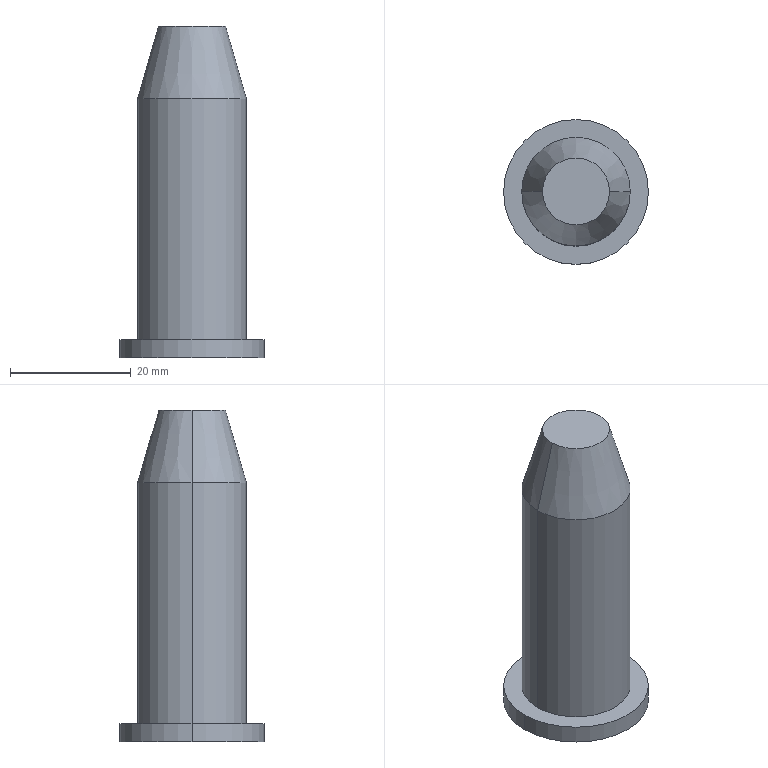Part | STEP file | YCD14007A-08.02.15 Latch Cylinder Joint | 1 solid | 13 faces | box 24 x 24 x 55 mm | volume 9061 mm3 | cylinder 6 | cone 4 | plane 3 | commonest cylinder face diameters 12.5 x2 18 x2 24 x2
STEP:
#1=CARTESIAN_POINT('',(0.,0.,0.));
#2=DIRECTION('',(0.,0.,1.));
#3=DIRECTION('',(1.,0.,0.));
#4=AXIS2_PLACEMENT_3D('',#1,#2,#3);
#5=CARTESIAN_POINT('',(-6.25,0.,35.5));
#6=VERTEX_POINT('',#5);
#7=CARTESIAN_POINT('',(-6.25,0.,0.));
#8=VERTEX_POINT('',#7);
#9=CARTESIAN_POINT('',(-6.25,0.,0.));
#10=DIRECTION('',(0.,0.,-1.));
#11=VECTOR('',#10,1.);
#12=LINE('',#9,#11);
#13=CARTESIAN_POINT('',(0.,0.,0.));
#14=DIRECTION('',(0.,0.,-1.));
#15=DIRECTION('',(-1.,0.,0.));
#16=AXIS2_PLACEMENT_3D('',#13,#14,#15);
#17=CYLINDRICAL_SURFACE('',#16,6.25);
#18=CARTESIAN_POINT('',(6.283,0.));
#19=DIRECTION('',(0.,1.));
#20=VECTOR('',#19,1.);
#21=LINE('',#18,#20);
#22=(GEOMETRIC_REPRESENTATION_CONTEXT(2)PARAMETRIC_REPRESENTATION_CONTEXT()REPRESENTATION_CONTEXT('',''));
#23=DEFINITIONAL_REPRESENTATION('',(#21),#22);
#24=PCURVE('',#17,#23);
#25=CARTESIAN_POINT('',(0.,0.,0.));
#26=DIRECTION('',(0.,0.,-1.));
#27=DIRECTION('',(-1.,0.,0.));
#28=AXIS2_PLACEMENT_3D('',#25,#26,#27);
#29=CYLINDRICAL_SURFACE('',#28,6.25);
#30=CARTESIAN_POINT('',(0.,0.));
#31=DIRECTION('',(0.,1.));
#32=VECTOR('',#31,1.);
#33=LINE('',#30,#32);
#34=(GEOMETRIC_REPRESENTATION_CONTEXT(2)PARAMETRIC_REPRESENTATION_CONTEXT()REPRESENTATION_CONTEXT('',''));
#35=DEFINITIONAL_REPRESENTATION('',(#33),#34);
#36=PCURVE('',#29,#35);
#37=SURFACE_CURVE('',#12,(#24,#36),.PCURVE_S1.);
#38=EDGE_CURVE('',#6,#8,#37,.T.);
#39=ORIENTED_EDGE('',*,*,#38,.T.);
#40=CARTESIAN_POINT('',(6.25,0.,0.));
#41=VERTEX_POINT('',#40);
#42=CARTESIAN_POINT('',(0.,0.,0.));
#43=DIRECTION('',(0.,0.,-1.));
#44=DIRECTION('',(-1.,0.,0.));
#45=AXIS2_PLACEMENT_3D('',#42,#43,#44);
#46=CIRCLE('',#45,6.25);
#47=CARTESIAN_POINT('',(0.,0.));
#48=DIRECTION('',(1.,0.));
#49=VECTOR('',#48,1.);
#50=LINE('',#47,#49);
#51=(GEOMETRIC_REPRESENTATION_CONTEXT(2)PARAMETRIC_REPRESENTATION_CONTEXT()REPRESENTATION_CONTEXT('',''));
#52=DEFINITIONAL_REPRESENTATION('',(#50),#51);
#53=PCURVE('',#17,#52);
#54=CARTESIAN_POINT('',(0.,0.,0.));
#55=DIRECTION('',(0.,0.,1.));
#56=DIRECTION('',(1.,0.,0.));
#57=AXIS2_PLACEMENT_3D('',#54,#55,#56);
#58=PLANE('',#57);
#59=CARTESIAN_POINT('',(-6.25,0.));
#60=CARTESIAN_POINT('',(-6.25,10.825));
#61=CARTESIAN_POINT('',(3.125,5.413));
#62=CARTESIAN_POINT('',(12.5,0.));
#63=CARTESIAN_POINT('',(3.125,-5.413));
#64=CARTESIAN_POINT('',(-6.25,-10.825));
#65=CARTESIAN_POINT('',(-6.25,0.));
#66=(BOUNDED_CURVE()B_SPLINE_CURVE(2,(#59,#60,#61,#62,#63,#64,#65),.UNSPECIFIED.,.T.,.F.)B_SPLINE_CURVE_WITH_KNOTS((1,2,2,2,2,1),(-2.094,0.,2.094,4.189,6.283,8.378),.UNSPECIFIED.)CURVE()GEOMETRIC_REPRESENTATION_ITEM()RATIONAL_B_SPLINE_CURVE((1.,0.5,1.,0.5,1.,0.5,1.))REPRESENTATION_ITEM(''));
#67=(GEOMETRIC_REPRESENTATION_CONTEXT(2)PARAMETRIC_REPRESENTATION_CONTEXT()REPRESENTATION_CONTEXT('',''));
#68=DEFINITIONAL_REPRESENTATION('',(#66),#67);
#69=PCURVE('',#58,#68);
#70=SURFACE_CURVE('',#46,(#53,#69),.PCURVE_S1.);
#71=EDGE_CURVE('',#41,#8,#70,.T.);
#72=ORIENTED_EDGE('',*,*,#71,.F.);
#73=CARTESIAN_POINT('',(6.25,0.,35.5));
#74=VERTEX_POINT('',#73);
#75=CARTESIAN_POINT('',(6.25,0.,0.));
#76=DIRECTION('',(0.,0.,-1.));
#77=VECTOR('',#76,1.);
#78=LINE('',#75,#77);
#79=CARTESIAN_POINT('',(3.142,0.));
#80=DIRECTION('',(0.,1.));
#81=VECTOR('',#80,1.);
#82=LINE('',#79,#81);
#83=(GEOMETRIC_REPRESENTATION_CONTEXT(2)PARAMETRIC_REPRESENTATION_CONTEXT()REPRESENTATION_CONTEXT('',''));
#84=DEFINITIONAL_REPRESENTATION('',(#82),#83);
#85=PCURVE('',#17,#84);
#86=CARTESIAN_POINT('',(3.142,0.));
#87=DIRECTION('',(0.,1.));
#88=VECTOR('',#87,1.);
#89=LINE('',#86,#88);
#90=(GEOMETRIC_REPRESENTATION_CONTEXT(2)PARAMETRIC_REPRESENTATION_CONTEXT()REPRESENTATION_CONTEXT('',''));
#91=DEFINITIONAL_REPRESENTATION('',(#89),#90);
#92=PCURVE('',#29,#91);
#93=SURFACE_CURVE('',#78,(#85,#92),.PCURVE_S1.);
#94=EDGE_CURVE('',#74,#41,#93,.T.);
#95=ORIENTED_EDGE('',*,*,#94,.F.);
#96=CARTESIAN_POINT('',(0.,0.,35.5));
#97=DIRECTION('',(0.,0.,-1.));
#98=DIRECTION('',(-1.,0.,0.));
#99=AXIS2_PLACEMENT_3D('',#96,#97,#98);
#100=CIRCLE('',#99,6.25);
#101=CARTESIAN_POINT('',(0.,-35.5));
#102=DIRECTION('',(1.,0.));
#103=VECTOR('',#102,1.);
#104=LINE('',#101,#103);
#105=(GEOMETRIC_REPRESENTATION_CONTEXT(2)PARAMETRIC_REPRESENTATION_CONTEXT()REPRESENTATION_CONTEXT('',''));
#106=DEFINITIONAL_REPRESENTATION('',(#104),#105);
#107=PCURVE('',#17,#106);
#108=CARTESIAN_POINT('',(0.,0.,35.5));
#109=DIRECTION('',(0.,0.,-1.));
#110=DIRECTION('',(-1.,0.,0.));
#111=AXIS2_PLACEMENT_3D('',#108,#109,#110);
#112=CONICAL_SURFACE('',#111,6.25,1.03);
#113=CARTESIAN_POINT('',(0.,0.));
#114=DIRECTION('',(1.,0.));
#115=VECTOR('',#114,1.);
#116=LINE('',#113,#115);
#117=(GEOMETRIC_REPRESENTATION_CONTEXT(2)PARAMETRIC_REPRESENTATION_CONTEXT()REPRESENTATION_CONTEXT('',''));
#118=DEFINITIONAL_REPRESENTATION('',(#116),#117);
#119=PCURVE('',#112,#118);
#120=SURFACE_CURVE('',#100,(#107,#119),.PCURVE_S1.);
#121=EDGE_CURVE('',#74,#6,#120,.T.);
#122=ORIENTED_EDGE('',*,*,#121,.T.);
#123=EDGE_LOOP('',(#39,#72,#95,#122));
#124=FACE_BOUND('',#123,.F.);
#125=ADVANCED_FACE('',(#124),#17,.F.);
#126=ORIENTED_EDGE('',*,*,#121,.F.);
#127=CARTESIAN_POINT('',(0.,0.,39.255));
#128=VERTEX_POINT('',#127);
#129=CARTESIAN_POINT('',(6.25,0.,35.5));
#130=DIRECTION('',(0.8572,0.,-0.515));
#131=VECTOR('',#130,1.);
#132=LINE('',#129,#131);
#133=CARTESIAN_POINT('',(3.142,-3.755));
#134=CARTESIAN_POINT('',(3.142,-3.698));
#135=CARTESIAN_POINT('',(3.142,-3.585));
#136=CARTESIAN_POINT('',(3.142,-3.414));
#137=CARTESIAN_POINT('',(3.142,-3.243));
#138=CARTESIAN_POINT('',(3.142,-3.073));
#139=CARTESIAN_POINT('',(3.142,-2.902));
#140=CARTESIAN_POINT('',(3.142,-2.731));
#141=CARTESIAN_POINT('',(3.142,-2.56));
#142=CARTESIAN_POINT('',(3.142,-2.39));
#143=CARTESIAN_POINT('',(3.142,-2.219));
#144=CARTESIAN_POINT('',(3.142,-2.048));
#145=CARTESIAN_POINT('',(3.142,-1.878));
#146=CARTESIAN_POINT('',(3.142,-1.707));
#147=CARTESIAN_POINT('',(3.142,-1.536));
#148=CARTESIAN_POINT('',(3.142,-1.366));
#149=CARTESIAN_POINT('',(3.142,-1.195));
#150=CARTESIAN_POINT('',(3.142,-1.024));
#151=CARTESIAN_POINT('',(3.142,-0.8535));
#152=CARTESIAN_POINT('',(3.142,-0.6828));
#153=CARTESIAN_POINT('',(3.142,-0.5121));
#154=CARTESIAN_POINT('',(3.142,-0.3414));
#155=CARTESIAN_POINT('',(3.142,-0.1707));
#156=CARTESIAN_POINT('',(3.142,-0.0569));
#157=CARTESIAN_POINT('',(3.142,0.));
#158=B_SPLINE_CURVE_WITH_KNOTS('',3,(#133,#134,#135,#136,#137,#138,#139,#140,#141,#142,#143,#144,#145,#146,#147,#148,#149,#150,#151,#152,#153,#154,#155,#156,#157),.UNSPECIFIED.,.F.,.F.,(4,1,1,1,1,1,1,1,1,1,1,1,1,1,1,1,1,1,1,1,1,1,4),(-7.291,-6.96,-6.629,-6.297,-5.966,-5.634,-5.303,-4.971,-4.64,-4.309,-3.977,-3.646,-3.314,-2.983,-2.651,-2.32,-1.989,-1.657,-1.326,-0.9943,-0.6629,-0.3314,0.),.UNSPECIFIED.);
#159=(GEOMETRIC_REPRESENTATION_CONTEXT(2)PARAMETRIC_REPRESENTATION_CONTEXT()REPRESENTATION_CONTEXT('',''));
#160=DEFINITIONAL_REPRESENTATION('',(#158),#159);
#161=PCURVE('',#112,#160);
#162=CARTESIAN_POINT('',(0.,0.,35.5));
#163=DIRECTION('',(0.,0.,-1.));
#164=DIRECTION('',(-1.,0.,0.));
#165=AXIS2_PLACEMENT_3D('',#162,#163,#164);
#166=CONICAL_SURFACE('',#165,6.25,1.03);
#167=CARTESIAN_POINT('',(3.142,-3.755));
#168=CARTESIAN_POINT('',(3.142,-3.698));
#169=CARTESIAN_POINT('',(3.142,-3.585));
#170=CARTESIAN_POINT('',(3.142,-3.414));
#171=CARTESIAN_POINT('',(3.142,-3.243));
#172=CARTESIAN_POINT('',(3.142,-3.073));
#173=CARTESIAN_POINT('',(3.142,-2.902));
#174=CARTESIAN_POINT('',(3.142,-2.731));
#175=CARTESIAN_POINT('',(3.142,-2.56));
#176=CARTESIAN_POINT('',(3.142,-2.39));
#177=CARTESIAN_POINT('',(3.142,-2.219));
#178=CARTESIAN_POINT('',(3.142,-2.048));
#179=CARTESIAN_POINT('',(3.142,-1.878));
#180=CARTESIAN_POINT('',(3.142,-1.707));
#181=CARTESIAN_POINT('',(3.142,-1.536));
#182=CARTESIAN_POINT('',(3.142,-1.366));
#183=CARTESIAN_POINT('',(3.142,-1.195));
#184=CARTESIAN_POINT('',(3.142,-1.024));
#185=CARTESIAN_POINT('',(3.142,-0.8535));
#186=CARTESIAN_POINT('',(3.142,-0.6828));
#187=CARTESIAN_POINT('',(3.142,-0.5121));
#188=CARTESIAN_POINT('',(3.142,-0.3414));
#189=CARTESIAN_POINT('',(3.142,-0.1707));
#190=CARTESIAN_POINT('',(3.142,-0.0569));
#191=CARTESIAN_POINT('',(3.142,0.));
#192=B_SPLINE_CURVE_WITH_KNOTS('',3,(#167,#168,#169,#170,#171,#172,#173,#174,#175,#176,#177,#178,#179,#180,#181,#182,#183,#184,#185,#186,#187,#188,#189,#190,#191),.UNSPECIFIED.,.F.,.F.,(4,1,1,1,1,1,1,1,1,1,1,1,1,1,1,1,1,1,1,1,1,1,4),(-7.291,-6.96,-6.629,-6.297,-5.966,-5.634,-5.303,-4.971,-4.64,-4.309,-3.977,-3.646,-3.314,-2.983,-2.651,-2.32,-1.989,-1.657,-1.326,-0.9943,-0.6629,-0.3314,0.),.UNSPECIFIED.);
#193=(GEOMETRIC_REPRESENTATION_CONTEXT(2)PARAMETRIC_REPRESENTATION_CONTEXT()REPRESENTATION_CONTEXT('',''));
#194=DEFINITIONAL_REPRESENTATION('',(#192),#193);
#195=PCURVE('',#166,#194);
#196=SURFACE_CURVE('',#132,(#161,#195),.PCURVE_S1.);
#197=EDGE_CURVE('',#128,#74,#196,.T.);
#198=ORIENTED_EDGE('',*,*,#197,.F.);
#199=CARTESIAN_POINT('',(-6.25,0.,35.5));
#200=DIRECTION('',(-0.8572,0.,-0.515));
#201=VECTOR('',#200,1.);
#202=LINE('',#199,#201);
#203=CARTESIAN_POINT('',(6.283,0.));
#204=DIRECTION('',(0.,1.));
#205=VECTOR('',#204,1.);
#206=LINE('',#203,#205);
#207=(GEOMETRIC_REPRESENTATION_CONTEXT(2)PARAMETRIC_REPRESENTATION_CONTEXT()REPRESENTATION_CONTEXT('',''));
#208=DEFINITIONAL_REPRESENTATION('',(#206),#207);
#209=PCURVE('',#112,#208);
#210=CARTESIAN_POINT('',(0.,0.));
#211=DIRECTION('',(0.,1.));
#212=VECTOR('',#211,1.);
#213=LINE('',#210,#212);
#214=(GEOMETRIC_REPRESENTATION_CONTEXT(2)PARAMETRIC_REPRESENTATION_CONTEXT()REPRESENTATION_CONTEXT('',''));
#215=DEFINITIONAL_REPRESENTATION('',(#213),#214);
#216=PCURVE('',#166,#215);
#217=SURFACE_CURVE('',#202,(#209,#216),.PCURVE_S1.);
#218=EDGE_CURVE('',#128,#6,#217,.T.);
#219=ORIENTED_EDGE('',*,*,#218,.T.);
#220=EDGE_LOOP('',(#126,#198,#219));
#221=FACE_BOUND('',#220,.F.);
#222=ADVANCED_FACE('',(#221),#112,.F.);
#223=CARTESIAN_POINT('',(5.559,0.,55.));
#224=VERTEX_POINT('',#223);
#225=CARTESIAN_POINT('',(-5.559,0.,55.));
#226=VERTEX_POINT('',#225);
#227=CARTESIAN_POINT('',(0.,0.,55.));
#228=DIRECTION('',(0.,0.,1.));
#229=DIRECTION('',(1.,0.,0.));
#230=AXIS2_PLACEMENT_3D('',#227,#228,#229);
#231=CIRCLE('',#230,5.559);
#232=CARTESIAN_POINT('',(0.,0.,55.));
#233=DIRECTION('',(0.,0.,-1.));
#234=DIRECTION('',(-1.,0.,0.));
#235=AXIS2_PLACEMENT_3D('',#232,#233,#234);
#236=CONICAL_SURFACE('',#235,5.559,0.2793);
#237=CARTESIAN_POINT('',(3.142,0.));
#238=DIRECTION('',(-1.,0.));
#239=VECTOR('',#238,1.);
#240=LINE('',#237,#239);
#241=(GEOMETRIC_REPRESENTATION_CONTEXT(2)PARAMETRIC_REPRESENTATION_CONTEXT()REPRESENTATION_CONTEXT('',''));
#242=DEFINITIONAL_REPRESENTATION('',(#240),#241);
#243=PCURVE('',#236,#242);
#244=CARTESIAN_POINT('',(0.,0.,55.));
#245=DIRECTION('',(0.,0.,1.));
#246=DIRECTION('',(1.,0.,0.));
#247=AXIS2_PLACEMENT_3D('',#244,#245,#246);
#248=PLANE('',#247);
#249=CARTESIAN_POINT('',(0.,0.));
#250=DIRECTION('',(1.,0.));
#251=AXIS2_PLACEMENT_2D('',#249,#250);
#252=CIRCLE('',#251,5.559);
#253=(GEOMETRIC_REPRESENTATION_CONTEXT(2)PARAMETRIC_REPRESENTATION_CONTEXT()REPRESENTATION_CONTEXT('',''));
#254=DEFINITIONAL_REPRESENTATION('',(#252),#253);
#255=PCURVE('',#248,#254);
#256=SURFACE_CURVE('',#231,(#243,#255),.PCURVE_S1.);
#257=EDGE_CURVE('',#224,#226,#256,.T.);
#258=ORIENTED_EDGE('',*,*,#257,.F.);
#259=CARTESIAN_POINT('',(9.,0.,43.));
#260=VERTEX_POINT('',#259);
#261=CARTESIAN_POINT('',(5.559,0.,55.));
#262=DIRECTION('',(0.2756,0.,-0.9613));
#263=VECTOR('',#262,1.);
#264=LINE('',#261,#263);
#265=CARTESIAN_POINT('',(3.142,0.));
#266=DIRECTION('',(0.,1.));
#267=VECTOR('',#266,1.);
#268=LINE('',#265,#267);
#269=(GEOMETRIC_REPRESENTATION_CONTEXT(2)PARAMETRIC_REPRESENTATION_CONTEXT()REPRESENTATION_CONTEXT('',''));
#270=DEFINITIONAL_REPRESENTATION('',(#268),#269);
#271=PCURVE('',#236,#270);
#272=CARTESIAN_POINT('',(0.,0.,55.));
#273=DIRECTION('',(0.,0.,-1.));
#274=DIRECTION('',(-1.,0.,0.));
#275=AXIS2_PLACEMENT_3D('',#272,#273,#274);
#276=CONICAL_SURFACE('',#275,5.559,0.2793);
#277=CARTESIAN_POINT('',(3.142,0.));
#278=DIRECTION('',(0.,1.));
#279=VECTOR('',#278,1.);
#280=LINE('',#277,#279);
#281=(GEOMETRIC_REPRESENTATION_CONTEXT(2)PARAMETRIC_REPRESENTATION_CONTEXT()REPRESENTATION_CONTEXT('',''));
#282=DEFINITIONAL_REPRESENTATION('',(#280),#281);
#283=PCURVE('',#276,#282);
#284=SURFACE_CURVE('',#264,(#271,#283),.PCURVE_S1.);
#285=EDGE_CURVE('',#224,#260,#284,.T.);
#286=ORIENTED_EDGE('',*,*,#285,.T.);
#287=CARTESIAN_POINT('',(-9.,0.,43.));
#288=VERTEX_POINT('',#287);
#289=CARTESIAN_POINT('',(0.,0.,43.));
#290=DIRECTION('',(0.,0.,-1.));
#291=DIRECTION('',(1.,0.,0.));
#292=AXIS2_PLACEMENT_3D('',#289,#290,#291);
#293=CIRCLE('',#292,9.);
#294=CARTESIAN_POINT('',(-3.142,12.));
#295=DIRECTION('',(1.,0.));
#296=VECTOR('',#295,1.);
#297=LINE('',#294,#296);
#298=(GEOMETRIC_REPRESENTATION_CONTEXT(2)PARAMETRIC_REPRESENTATION_CONTEXT()REPRESENTATION_CONTEXT('',''));
#299=DEFINITIONAL_REPRESENTATION('',(#297),#298);
#300=PCURVE('',#236,#299);
#301=CARTESIAN_POINT('',(0.,0.,55.));
#302=DIRECTION('',(0.,0.,-1.));
#303=DIRECTION('',(-1.,0.,0.));
#304=AXIS2_PLACEMENT_3D('',#301,#302,#303);
#305=CYLINDRICAL_SURFACE('',#304,9.);
#306=CARTESIAN_POINT('',(-3.142,12.));
#307=DIRECTION('',(1.,0.));
#308=VECTOR('',#307,1.);
#309=LINE('',#306,#308);
#310=(GEOMETRIC_REPRESENTATION_CONTEXT(2)PARAMETRIC_REPRESENTATION_CONTEXT()REPRESENTATION_CONTEXT('',''));
#311=DEFINITIONAL_REPRESENTATION('',(#309),#310);
#312=PCURVE('',#305,#311);
#313=SURFACE_CURVE('',#293,(#300,#312),.PCURVE_S1.);
#314=EDGE_CURVE('',#288,#260,#313,.T.);
#315=ORIENTED_EDGE('',*,*,#314,.F.);
#316=CARTESIAN_POINT('',(-5.559,0.,55.));
#317=DIRECTION('',(-0.2756,0.,-0.9613));
#318=VECTOR('',#317,1.);
#319=LINE('',#316,#318);
#320=CARTESIAN_POINT('',(0.,0.));
#321=DIRECTION('',(0.,1.));
#322=VECTOR('',#321,1.);
#323=LINE('',#320,#322);
#324=(GEOMETRIC_REPRESENTATION_CONTEXT(2)PARAMETRIC_REPRESENTATION_CONTEXT()REPRESENTATION_CONTEXT('',''));
#325=DEFINITIONAL_REPRESENTATION('',(#323),#324);
#326=PCURVE('',#236,#325);
#327=CARTESIAN_POINT('',(6.283,0.));
#328=DIRECTION('',(0.,1.));
#329=VECTOR('',#328,1.);
#330=LINE('',#327,#329);
#331=(GEOMETRIC_REPRESENTATION_CONTEXT(2)PARAMETRIC_REPRESENTATION_CONTEXT()REPRESENTATION_CONTEXT('',''));
#332=DEFINITIONAL_REPRESENTATION('',(#330),#331);
#333=PCURVE('',#276,#332);
#334=SURFACE_CURVE('',#319,(#326,#333),.PCURVE_S1.);
#335=EDGE_CURVE('',#226,#288,#334,.T.);
#336=ORIENTED_EDGE('',*,*,#335,.F.);
#337=EDGE_LOOP('',(#258,#286,#315,#336));
#338=FACE_BOUND('',#337,.T.);
#339=ADVANCED_FACE('',(#338),#236,.T.);
#340=ORIENTED_EDGE('',*,*,#314,.T.);
#341=CARTESIAN_POINT('',(9.,0.,3.));
#342=VERTEX_POINT('',#341);
#343=CARTESIAN_POINT('',(9.,0.,55.));
#344=DIRECTION('',(0.,0.,-1.));
#345=VECTOR('',#344,1.);
#346=LINE('',#343,#345);
#347=CARTESIAN_POINT('',(3.142,0.));
#348=DIRECTION('',(0.,1.));
#349=VECTOR('',#348,1.);
#350=LINE('',#347,#349);
#351=(GEOMETRIC_REPRESENTATION_CONTEXT(2)PARAMETRIC_REPRESENTATION_CONTEXT()REPRESENTATION_CONTEXT('',''));
#352=DEFINITIONAL_REPRESENTATION('',(#350),#351);
#353=PCURVE('',#305,#352);
#354=CARTESIAN_POINT('',(0.,0.,55.));
#355=DIRECTION('',(0.,0.,-1.));
#356=DIRECTION('',(-1.,0.,0.));
#357=AXIS2_PLACEMENT_3D('',#354,#355,#356);
#358=CYLINDRICAL_SURFACE('',#357,9.);
#359=CARTESIAN_POINT('',(3.142,0.));
#360=DIRECTION('',(0.,1.));
#361=VECTOR('',#360,1.);
#362=LINE('',#359,#361);
#363=(GEOMETRIC_REPRESENTATION_CONTEXT(2)PARAMETRIC_REPRESENTATION_CONTEXT()REPRESENTATION_CONTEXT('',''));
#364=DEFINITIONAL_REPRESENTATION('',(#362),#363);
#365=PCURVE('',#358,#364);
#366=SURFACE_CURVE('',#346,(#353,#365),.PCURVE_S1.);
#367=EDGE_CURVE('',#260,#342,#366,.T.);
#368=ORIENTED_EDGE('',*,*,#367,.T.);
#369=CARTESIAN_POINT('',(-9.,0.,3.));
#370=VERTEX_POINT('',#369);
#371=CARTESIAN_POINT('',(0.,0.,3.));
#372=DIRECTION('',(0.,0.,1.));
#373=DIRECTION('',(1.,0.,0.));
#374=AXIS2_PLACEMENT_3D('',#371,#372,#373);
#375=CIRCLE('',#374,9.);
#376=CARTESIAN_POINT('',(3.142,52.));
#377=DIRECTION('',(-1.,0.));
#378=VECTOR('',#377,1.);
#379=LINE('',#376,#378);
#380=(GEOMETRIC_REPRESENTATION_CONTEXT(2)PARAMETRIC_REPRESENTATION_CONTEXT()REPRESENTATION_CONTEXT('',''));
#381=DEFINITIONAL_REPRESENTATION('',(#379),#380);
#382=PCURVE('',#305,#381);
#383=CARTESIAN_POINT('',(0.,0.,3.));
#384=DIRECTION('',(0.,0.,1.));
#385=DIRECTION('',(1.,0.,0.));
#386=AXIS2_PLACEMENT_3D('',#383,#384,#385);
#387=PLANE('',#386);
#388=CARTESIAN_POINT('',(0.,0.));
#389=DIRECTION('',(1.,0.));
#390=AXIS2_PLACEMENT_2D('',#388,#389);
#391=CIRCLE('',#390,9.);
#392=(GEOMETRIC_REPRESENTATION_CONTEXT(2)PARAMETRIC_REPRESENTATION_CONTEXT()REPRESENTATION_CONTEXT('',''));
#393=DEFINITIONAL_REPRESENTATION('',(#391),#392);
#394=PCURVE('',#387,#393);
#395=SURFACE_CURVE('',#375,(#382,#394),.PCURVE_S1.);
#396=EDGE_CURVE('',#342,#370,#395,.T.);
#397=ORIENTED_EDGE('',*,*,#396,.T.);
#398=CARTESIAN_POINT('',(-9.,0.,55.));
#399=DIRECTION('',(0.,0.,-1.));
#400=VECTOR('',#399,1.);
#401=LINE('',#398,#400);
#402=CARTESIAN_POINT('',(0.,0.));
#403=DIRECTION('',(0.,1.));
#404=VECTOR('',#403,1.);
#405=LINE('',#402,#404);
#406=(GEOMETRIC_REPRESENTATION_CONTEXT(2)PARAMETRIC_REPRESENTATION_CONTEXT()REPRESENTATION_CONTEXT('',''));
#407=DEFINITIONAL_REPRESENTATION('',(#405),#406);
#408=PCURVE('',#305,#407);
#409=CARTESIAN_POINT('',(6.283,0.));
#410=DIRECTION('',(0.,1.));
#411=VECTOR('',#410,1.);
#412=LINE('',#409,#411);
#413=(GEOMETRIC_REPRESENTATION_CONTEXT(2)PARAMETRIC_REPRESENTATION_CONTEXT()REPRESENTATION_CONTEXT('',''));
#414=DEFINITIONAL_REPRESENTATION('',(#412),#413);
#415=PCURVE('',#358,#414);
#416=SURFACE_CURVE('',#401,(#408,#415),.PCURVE_S1.);
#417=EDGE_CURVE('',#288,#370,#416,.T.);
#418=ORIENTED_EDGE('',*,*,#417,.F.);
#419=EDGE_LOOP('',(#340,#368,#397,#418));
#420=FACE_BOUND('',#419,.T.);
#421=ADVANCED_FACE('',(#420),#305,.T.);
#422=CARTESIAN_POINT('',(12.,0.,3.));
#423=VERTEX_POINT('',#422);
#424=CARTESIAN_POINT('',(-12.,0.,3.));
#425=VERTEX_POINT('',#424);
#426=CARTESIAN_POINT('',(0.,0.,3.));
#427=DIRECTION('',(0.,0.,1.));
#428=DIRECTION('',(1.,0.,0.));
#429=AXIS2_PLACEMENT_3D('',#426,#427,#428);
#430=CIRCLE('',#429,12.);
#431=CARTESIAN_POINT('',(0.,0.,3.));
#432=DIRECTION('',(0.,0.,-1.));
#433=DIRECTION('',(-1.,0.,0.));
#434=AXIS2_PLACEMENT_3D('',#431,#432,#433);
#435=CYLINDRICAL_SURFACE('',#434,12.);
#436=CARTESIAN_POINT('',(3.142,0.));
#437=DIRECTION('',(-1.,0.));
#438=VECTOR('',#437,1.);
#439=LINE('',#436,#438);
#440=(GEOMETRIC_REPRESENTATION_CONTEXT(2)PARAMETRIC_REPRESENTATION_CONTEXT()REPRESENTATION_CONTEXT('',''));
#441=DEFINITIONAL_REPRESENTATION('',(#439),#440);
#442=PCURVE('',#435,#441);
#443=CARTESIAN_POINT('',(0.,0.));
#444=DIRECTION('',(1.,0.));
#445=AXIS2_PLACEMENT_2D('',#443,#444);
#446=CIRCLE('',#445,12.);
#447=(GEOMETRIC_REPRESENTATION_CONTEXT(2)PARAMETRIC_REPRESENTATION_CONTEXT()REPRESENTATION_CONTEXT('',''));
#448=DEFINITIONAL_REPRESENTATION('',(#446),#447);
#449=PCURVE('',#387,#448);
#450=SURFACE_CURVE('',#430,(#442,#449),.PCURVE_S1.);
#451=EDGE_CURVE('',#423,#425,#450,.T.);
#452=ORIENTED_EDGE('',*,*,#451,.F.);
#453=CARTESIAN_POINT('',(12.,0.,0.));
#454=VERTEX_POINT('',#453);
#455=CARTESIAN_POINT('',(12.,0.,3.));
#456=DIRECTION('',(0.,0.,-1.));
#457=VECTOR('',#456,1.);
#458=LINE('',#455,#457);
#459=CARTESIAN_POINT('',(3.142,0.));
#460=DIRECTION('',(0.,1.));
#461=VECTOR('',#460,1.);
#462=LINE('',#459,#461);
#463=(GEOMETRIC_REPRESENTATION_CONTEXT(2)PARAMETRIC_REPRESENTATION_CONTEXT()REPRESENTATION_CONTEXT('',''));
#464=DEFINITIONAL_REPRESENTATION('',(#462),#463);
#465=PCURVE('',#435,#464);
#466=CARTESIAN_POINT('',(0.,0.,3.));
#467=DIRECTION('',(0.,0.,-1.));
#468=DIRECTION('',(-1.,0.,0.));
#469=AXIS2_PLACEMENT_3D('',#466,#467,#468);
#470=CYLINDRICAL_SURFACE('',#469,12.);
#471=CARTESIAN_POINT('',(3.142,0.));
#472=DIRECTION('',(0.,1.));
#473=VECTOR('',#472,1.);
#474=LINE('',#471,#473);
#475=(GEOMETRIC_REPRESENTATION_CONTEXT(2)PARAMETRIC_REPRESENTATION_CONTEXT()REPRESENTATION_CONTEXT('',''));
#476=DEFINITIONAL_REPRESENTATION('',(#474),#475);
#477=PCURVE('',#470,#476);
#478=SURFACE_CURVE('',#458,(#465,#477),.PCURVE_S1.);
#479=EDGE_CURVE('',#423,#454,#478,.T.);
#480=ORIENTED_EDGE('',*,*,#479,.T.);
#481=CARTESIAN_POINT('',(-12.,0.,0.));
#482=VERTEX_POINT('',#481);
#483=CARTESIAN_POINT('',(0.,0.,0.));
#484=DIRECTION('',(0.,0.,1.));
#485=DIRECTION('',(1.,0.,0.));
#486=AXIS2_PLACEMENT_3D('',#483,#484,#485);
#487=CIRCLE('',#486,12.);
#488=CARTESIAN_POINT('',(3.142,3.));
#489=DIRECTION('',(-1.,0.));
#490=VECTOR('',#489,1.);
#491=LINE('',#488,#490);
#492=(GEOMETRIC_REPRESENTATION_CONTEXT(2)PARAMETRIC_REPRESENTATION_CONTEXT()REPRESENTATION_CONTEXT('',''));
#493=DEFINITIONAL_REPRESENTATION('',(#491),#492);
#494=PCURVE('',#435,#493);
#495=CARTESIAN_POINT('',(0.,0.));
#496=DIRECTION('',(1.,0.));
#497=AXIS2_PLACEMENT_2D('',#495,#496);
#498=CIRCLE('',#497,12.);
#499=(GEOMETRIC_REPRESENTATION_CONTEXT(2)PARAMETRIC_REPRESENTATION_CONTEXT()REPRESENTATION_CONTEXT('',''));
#500=DEFINITIONAL_REPRESENTATION('',(#498),#499);
#501=PCURVE('',#58,#500);
#502=SURFACE_CURVE('',#487,(#494,#501),.PCURVE_S1.);
#503=EDGE_CURVE('',#454,#482,#502,.T.);
#504=ORIENTED_EDGE('',*,*,#503,.T.);
#505=CARTESIAN_POINT('',(-12.,0.,3.));
#506=DIRECTION('',(0.,0.,-1.));
#507=VECTOR('',#506,1.);
#508=LINE('',#505,#507);
#509=CARTESIAN_POINT('',(0.,0.));
#510=DIRECTION('',(0.,1.));
#511=VECTOR('',#510,1.);
#512=LINE('',#509,#511);
#513=(GEOMETRIC_REPRESENTATION_CONTEXT(2)PARAMETRIC_REPRESENTATION_CONTEXT()REPRESENTATION_CONTEXT('',''));
#514=DEFINITIONAL_REPRESENTATION('',(#512),#513);
#515=PCURVE('',#435,#514);
#516=CARTESIAN_POINT('',(6.283,0.));
#517=DIRECTION('',(0.,1.));
#518=VECTOR('',#517,1.);
#519=LINE('',#516,#518);
#520=(GEOMETRIC_REPRESENTATION_CONTEXT(2)PARAMETRIC_REPRESENTATION_CONTEXT()REPRESENTATION_CONTEXT('',''));
#521=DEFINITIONAL_REPRESENTATION('',(#519),#520);
#522=PCURVE('',#470,#521);
#523=SURFACE_CURVE('',#508,(#515,#522),.PCURVE_S1.);
#524=EDGE_CURVE('',#425,#482,#523,.T.);
#525=ORIENTED_EDGE('',*,*,#524,.F.);
#526=EDGE_LOOP('',(#452,#480,#504,#525));
#527=FACE_BOUND('',#526,.T.);
#528=ADVANCED_FACE('',(#527),#435,.T.);
#529=CARTESIAN_POINT('',(0.,0.,3.));
#530=DIRECTION('',(0.,0.,1.));
#531=DIRECTION('',(1.,0.,0.));
#532=AXIS2_PLACEMENT_3D('',#529,#530,#531);
#533=CIRCLE('',#532,12.);
#534=CARTESIAN_POINT('',(0.,0.));
#535=DIRECTION('',(1.,0.));
#536=AXIS2_PLACEMENT_2D('',#534,#535);
#537=CIRCLE('',#536,12.);
#538=(GEOMETRIC_REPRESENTATION_CONTEXT(2)PARAMETRIC_REPRESENTATION_CONTEXT()REPRESENTATION_CONTEXT('',''));
#539=DEFINITIONAL_REPRESENTATION('',(#537),#538);
#540=PCURVE('',#387,#539);
#541=CARTESIAN_POINT('',(9.425,0.));
#542=DIRECTION('',(-1.,0.));
#543=VECTOR('',#542,1.);
#544=LINE('',#541,#543);
#545=(GEOMETRIC_REPRESENTATION_CONTEXT(2)PARAMETRIC_REPRESENTATION_CONTEXT()REPRESENTATION_CONTEXT('',''));
#546=DEFINITIONAL_REPRESENTATION('',(#544),#545);
#547=PCURVE('',#470,#546);
#548=SURFACE_CURVE('',#533,(#540,#547),.PCURVE_S1.);
#549=EDGE_CURVE('',#425,#423,#548,.T.);
#550=ORIENTED_EDGE('',*,*,#549,.T.);
#551=ORIENTED_EDGE('',*,*,#451,.T.);
#552=EDGE_LOOP('',(#550,#551));
#553=FACE_BOUND('',#552,.T.);
#554=CARTESIAN_POINT('',(0.,0.,3.));
#555=DIRECTION('',(0.,0.,1.));
#556=DIRECTION('',(1.,0.,0.));
#557=AXIS2_PLACEMENT_3D('',#554,#555,#556);
#558=CIRCLE('',#557,9.);
#559=CARTESIAN_POINT('',(0.,0.));
#560=DIRECTION('',(1.,0.));
#561=AXIS2_PLACEMENT_2D('',#559,#560);
#562=CIRCLE('',#561,9.);
#563=(GEOMETRIC_REPRESENTATION_CONTEXT(2)PARAMETRIC_REPRESENTATION_CONTEXT()REPRESENTATION_CONTEXT('',''));
#564=DEFINITIONAL_REPRESENTATION('',(#562),#563);
#565=PCURVE('',#387,#564);
#566=CARTESIAN_POINT('',(9.425,52.));
#567=DIRECTION('',(-1.,0.));
#568=VECTOR('',#567,1.);
#569=LINE('',#566,#568);
#570=(GEOMETRIC_REPRESENTATION_CONTEXT(2)PARAMETRIC_REPRESENTATION_CONTEXT()REPRESENTATION_CONTEXT('',''));
#571=DEFINITIONAL_REPRESENTATION('',(#569),#570);
#572=PCURVE('',#358,#571);
#573=SURFACE_CURVE('',#558,(#565,#572),.PCURVE_S1.);
#574=EDGE_CURVE('',#370,#342,#573,.T.);
#575=ORIENTED_EDGE('',*,*,#574,.F.);
#576=ORIENTED_EDGE('',*,*,#396,.F.);
#577=EDGE_LOOP('',(#575,#576));
#578=FACE_BOUND('',#577,.T.);
#579=ADVANCED_FACE('',(#553,#578),#387,.T.);
#580=ORIENTED_EDGE('',*,*,#479,.F.);
#581=ORIENTED_EDGE('',*,*,#549,.F.);
#582=ORIENTED_EDGE('',*,*,#524,.T.);
#583=CARTESIAN_POINT('',(0.,0.,0.));
#584=DIRECTION('',(0.,0.,1.));
#585=DIRECTION('',(1.,0.,0.));
#586=AXIS2_PLACEMENT_3D('',#583,#584,#585);
#587=CIRCLE('',#586,12.);
#588=CARTESIAN_POINT('',(9.425,3.));
#589=DIRECTION('',(-1.,0.));
#590=VECTOR('',#589,1.);
#591=LINE('',#588,#590);
#592=(GEOMETRIC_REPRESENTATION_CONTEXT(2)PARAMETRIC_REPRESENTATION_CONTEXT()REPRESENTATION_CONTEXT('',''));
#593=DEFINITIONAL_REPRESENTATION('',(#591),#592);
#594=PCURVE('',#470,#593);
#595=CARTESIAN_POINT('',(0.,0.));
#596=DIRECTION('',(1.,0.));
#597=AXIS2_PLACEMENT_2D('',#595,#596);
#598=CIRCLE('',#597,12.);
#599=(GEOMETRIC_REPRESENTATION_CONTEXT(2)PARAMETRIC_REPRESENTATION_CONTEXT()REPRESENTATION_CONTEXT('',''));
#600=DEFINITIONAL_REPRESENTATION('',(#598),#599);
#601=PCURVE('',#58,#600);
#602=SURFACE_CURVE('',#587,(#594,#601),.PCURVE_S1.);
#603=EDGE_CURVE('',#482,#454,#602,.T.);
#604=ORIENTED_EDGE('',*,*,#603,.T.);
#605=EDGE_LOOP('',(#580,#581,#582,#604));
#606=FACE_BOUND('',#605,.T.);
#607=ADVANCED_FACE('',(#606),#470,.T.);
#608=CARTESIAN_POINT('',(0.,0.,0.));
#609=DIRECTION('',(0.,0.,-1.));
#610=DIRECTION('',(-1.,0.,0.));
#611=AXIS2_PLACEMENT_3D('',#608,#609,#610);
#612=CIRCLE('',#611,6.25);
#613=CARTESIAN_POINT('',(-6.25,0.));
#614=CARTESIAN_POINT('',(-6.25,10.825));
#615=CARTESIAN_POINT('',(3.125,5.413));
#616=CARTESIAN_POINT('',(12.5,0.));
#617=CARTESIAN_POINT('',(3.125,-5.413));
#618=CARTESIAN_POINT('',(-6.25,-10.825));
#619=CARTESIAN_POINT('',(-6.25,0.));
#620=(BOUNDED_CURVE()B_SPLINE_CURVE(2,(#613,#614,#615,#616,#617,#618,#619),.UNSPECIFIED.,.T.,.F.)B_SPLINE_CURVE_WITH_KNOTS((1,2,2,2,2,1),(-2.094,0.,2.094,4.189,6.283,8.378),.UNSPECIFIED.)CURVE()GEOMETRIC_REPRESENTATION_ITEM()RATIONAL_B_SPLINE_CURVE((1.,0.5,1.,0.5,1.,0.5,1.))REPRESENTATION_ITEM(''));
#621=(GEOMETRIC_REPRESENTATION_CONTEXT(2)PARAMETRIC_REPRESENTATION_CONTEXT()REPRESENTATION_CONTEXT('',''));
#622=DEFINITIONAL_REPRESENTATION('',(#620),#621);
#623=PCURVE('',#58,#622);
#624=CARTESIAN_POINT('',(0.,0.));
#625=DIRECTION('',(1.,0.));
#626=VECTOR('',#625,1.);
#627=LINE('',#624,#626);
#628=(GEOMETRIC_REPRESENTATION_CONTEXT(2)PARAMETRIC_REPRESENTATION_CONTEXT()REPRESENTATION_CONTEXT('',''));
#629=DEFINITIONAL_REPRESENTATION('',(#627),#628);
#630=PCURVE('',#29,#629);
#631=SURFACE_CURVE('',#612,(#623,#630),.PCURVE_S1.);
#632=EDGE_CURVE('',#8,#41,#631,.T.);
#633=ORIENTED_EDGE('',*,*,#632,.F.);
#634=ORIENTED_EDGE('',*,*,#71,.F.);
#635=EDGE_LOOP('',(#633,#634));
#636=FACE_BOUND('',#635,.T.);
#637=ORIENTED_EDGE('',*,*,#603,.F.);
#638=ORIENTED_EDGE('',*,*,#503,.F.);
#639=EDGE_LOOP('',(#637,#638));
#640=FACE_BOUND('',#639,.T.);
#641=ADVANCED_FACE('',(#636,#640),#58,.F.);
#642=ORIENTED_EDGE('',*,*,#367,.F.);
#643=CARTESIAN_POINT('',(0.,0.,43.));
#644=DIRECTION('',(0.,0.,-1.));
#645=DIRECTION('',(1.,0.,0.));
#646=AXIS2_PLACEMENT_3D('',#643,#644,#645);
#647=CIRCLE('',#646,9.);
#648=CARTESIAN_POINT('',(3.142,12.));
#649=DIRECTION('',(1.,0.));
#650=VECTOR('',#649,1.);
#651=LINE('',#648,#650);
#652=(GEOMETRIC_REPRESENTATION_CONTEXT(2)PARAMETRIC_REPRESENTATION_CONTEXT()REPRESENTATION_CONTEXT('',''));
#653=DEFINITIONAL_REPRESENTATION('',(#651),#652);
#654=PCURVE('',#358,#653);
#655=CARTESIAN_POINT('',(3.142,12.));
#656=DIRECTION('',(1.,0.));
#657=VECTOR('',#656,1.);
#658=LINE('',#655,#657);
#659=(GEOMETRIC_REPRESENTATION_CONTEXT(2)PARAMETRIC_REPRESENTATION_CONTEXT()REPRESENTATION_CONTEXT('',''));
#660=DEFINITIONAL_REPRESENTATION('',(#658),#659);
#661=PCURVE('',#276,#660);
#662=SURFACE_CURVE('',#647,(#654,#661),.PCURVE_S1.);
#663=EDGE_CURVE('',#260,#288,#662,.T.);
#664=ORIENTED_EDGE('',*,*,#663,.T.);
#665=ORIENTED_EDGE('',*,*,#417,.T.);
#666=ORIENTED_EDGE('',*,*,#574,.T.);
#667=EDGE_LOOP('',(#642,#664,#665,#666));
#668=FACE_BOUND('',#667,.T.);
#669=ADVANCED_FACE('',(#668),#358,.T.);
#670=CARTESIAN_POINT('',(0.,0.,55.));
#671=DIRECTION('',(0.,0.,1.));
#672=DIRECTION('',(1.,0.,0.));
#673=AXIS2_PLACEMENT_3D('',#670,#671,#672);
#674=CIRCLE('',#673,5.559);
#675=CARTESIAN_POINT('',(0.,0.));
#676=DIRECTION('',(1.,0.));
#677=AXIS2_PLACEMENT_2D('',#675,#676);
#678=CIRCLE('',#677,5.559);
#679=(GEOMETRIC_REPRESENTATION_CONTEXT(2)PARAMETRIC_REPRESENTATION_CONTEXT()REPRESENTATION_CONTEXT('',''));
#680=DEFINITIONAL_REPRESENTATION('',(#678),#679);
#681=PCURVE('',#248,#680);
#682=CARTESIAN_POINT('',(9.425,0.));
#683=DIRECTION('',(-1.,0.));
#684=VECTOR('',#683,1.);
#685=LINE('',#682,#684);
#686=(GEOMETRIC_REPRESENTATION_CONTEXT(2)PARAMETRIC_REPRESENTATION_CONTEXT()REPRESENTATION_CONTEXT('',''));
#687=DEFINITIONAL_REPRESENTATION('',(#685),#686);
#688=PCURVE('',#276,#687);
#689=SURFACE_CURVE('',#674,(#681,#688),.PCURVE_S1.);
#690=EDGE_CURVE('',#226,#224,#689,.T.);
#691=ORIENTED_EDGE('',*,*,#690,.T.);
#692=ORIENTED_EDGE('',*,*,#257,.T.);
#693=EDGE_LOOP('',(#691,#692));
#694=FACE_BOUND('',#693,.T.);
#695=ADVANCED_FACE('',(#694),#248,.T.);
#696=ORIENTED_EDGE('',*,*,#285,.F.);
#697=ORIENTED_EDGE('',*,*,#690,.F.);
#698=ORIENTED_EDGE('',*,*,#335,.T.);
#699=ORIENTED_EDGE('',*,*,#663,.F.);
#700=EDGE_LOOP('',(#696,#697,#698,#699));
#701=FACE_BOUND('',#700,.T.);
#702=ADVANCED_FACE('',(#701),#276,.T.);
#703=CARTESIAN_POINT('',(0.,0.,35.5));
#704=DIRECTION('',(0.,0.,-1.));
#705=DIRECTION('',(-1.,0.,0.));
#706=AXIS2_PLACEMENT_3D('',#703,#704,#705);
#707=CIRCLE('',#706,6.25);
#708=CARTESIAN_POINT('',(0.,0.));
#709=DIRECTION('',(1.,0.));
#710=VECTOR('',#709,1.);
#711=LINE('',#708,#710);
#712=(GEOMETRIC_REPRESENTATION_CONTEXT(2)PARAMETRIC_REPRESENTATION_CONTEXT()REPRESENTATION_CONTEXT('',''));
#713=DEFINITIONAL_REPRESENTATION('',(#711),#712);
#714=PCURVE('',#166,#713);
#715=CARTESIAN_POINT('',(0.,-35.5));
#716=DIRECTION('',(1.,0.));
#717=VECTOR('',#716,1.);
#718=LINE('',#715,#717);
#719=(GEOMETRIC_REPRESENTATION_CONTEXT(2)PARAMETRIC_REPRESENTATION_CONTEXT()REPRESENTATION_CONTEXT('',''));
#720=DEFINITIONAL_REPRESENTATION('',(#718),#719);
#721=PCURVE('',#29,#720);
#722=SURFACE_CURVE('',#707,(#714,#721),.PCURVE_S1.);
#723=EDGE_CURVE('',#6,#74,#722,.T.);
#724=ORIENTED_EDGE('',*,*,#723,.F.);
#725=ORIENTED_EDGE('',*,*,#218,.F.);
#726=ORIENTED_EDGE('',*,*,#197,.T.);
#727=EDGE_LOOP('',(#724,#725,#726));
#728=FACE_BOUND('',#727,.F.);
#729=ADVANCED_FACE('',(#728),#166,.F.);
#730=ORIENTED_EDGE('',*,*,#632,.F.);
#731=ORIENTED_EDGE('',*,*,#38,.F.);
#732=ORIENTED_EDGE('',*,*,#723,.T.);
#733=ORIENTED_EDGE('',*,*,#94,.T.);
#734=EDGE_LOOP('',(#730,#731,#732,#733));
#735=FACE_BOUND('',#734,.F.);
#736=ADVANCED_FACE('',(#735),#29,.F.);
#737=CLOSED_SHELL('',(#125,#222,#339,#421,#528,#579,#607,#641,#669,#695,#702,#729,#736));
#738=MANIFOLD_SOLID_BREP('',#737);
#739=(LENGTH_UNIT()NAMED_UNIT(*)SI_UNIT(.MILLI.,.METRE.));
#740=UNCERTAINTY_MEASURE_WITH_UNIT(LENGTH_MEASURE(0.0000001),#739,'','');
#741=(NAMED_UNIT(*)PLANE_ANGLE_UNIT()SI_UNIT($,.RADIAN.));
#742=(NAMED_UNIT(*)SI_UNIT($,.STERADIAN.)SOLID_ANGLE_UNIT());
#743=(GEOMETRIC_REPRESENTATION_CONTEXT(3)GLOBAL_UNCERTAINTY_ASSIGNED_CONTEXT((#740))GLOBAL_UNIT_ASSIGNED_CONTEXT((#739,#741,#742))REPRESENTATION_CONTEXT('',''));
#744=ADVANCED_BREP_SHAPE_REPRESENTATION('',(#4,#738),#743);